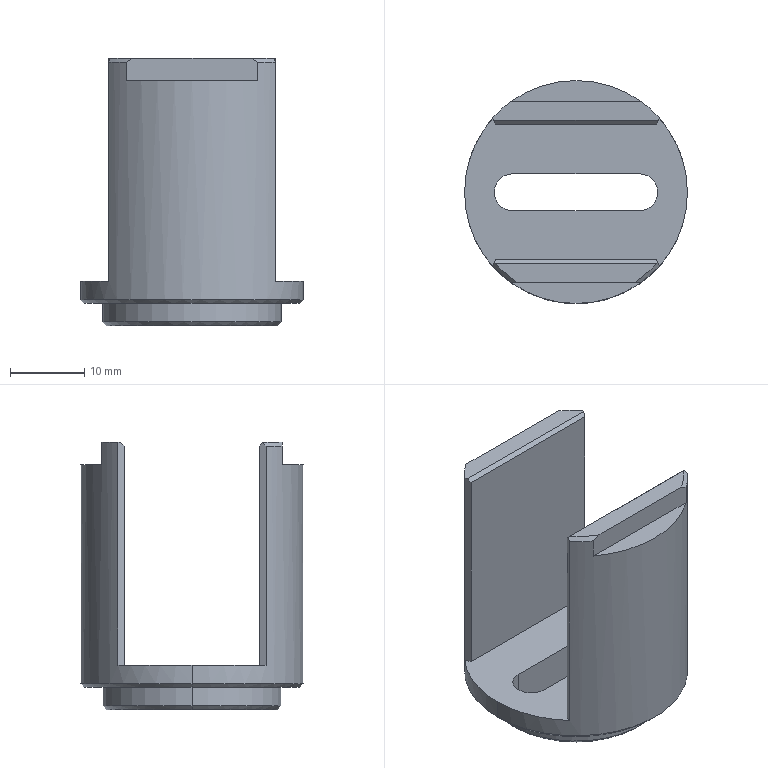Part | Creo | features CURVE 5, CHAMFER 3, DATUM PLANE 3, PROTRUSION 3, CUT 2, COORDINATE SYSTEM 1 | 1 solid | 31 faces | box 30 x 30 x 36 mm | volume 8414 mm3 | plane 19 | cylinder 6 | cone 6 | commonest cylinder face diameters 5 x2 24 x2 30 x2
STEP:
#1=CARTESIAN_POINT('',(0.,0.,0.));
#2=DIRECTION('',(0.,0.,1.));
#3=DIRECTION('',(1.,0.,0.));
#4=AXIS2_PLACEMENT_3D('',#1,#2,#3);
#5=CARTESIAN_POINT('',(-14.5,0.,0.));
#6=VERTEX_POINT('',#5);
#7=CARTESIAN_POINT('',(14.5,0.,0.));
#8=VERTEX_POINT('',#7);
#9=CARTESIAN_POINT('',(0.,0.,0.));
#10=DIRECTION('',(0.,0.,-1.));
#11=DIRECTION('',(-1.,0.,0.));
#12=AXIS2_PLACEMENT_3D('',#9,#10,#11);
#13=CIRCLE('',#12,14.5);
#14=EDGE_CURVE('',#6,#8,#13,.T.);
#15=ORIENTED_EDGE('',*,*,#14,.F.);
#16=CARTESIAN_POINT('',(0.,0.,0.));
#17=DIRECTION('',(0.,0.,-1.));
#18=DIRECTION('',(1.,0.,0.));
#19=AXIS2_PLACEMENT_3D('',#16,#17,#18);
#20=CIRCLE('',#19,14.5);
#21=EDGE_CURVE('',#8,#6,#20,.T.);
#22=ORIENTED_EDGE('',*,*,#21,.F.);
#23=EDGE_LOOP('',(#15,#22));
#24=FACE_OUTER_BOUND('',#23,.F.);
#25=CARTESIAN_POINT('',(12.,0.,0.));
#26=VERTEX_POINT('',#25);
#27=CARTESIAN_POINT('',(-12.,0.,0.));
#28=VERTEX_POINT('',#27);
#29=CARTESIAN_POINT('',(0.,0.,0.));
#30=DIRECTION('',(0.,0.,-1.));
#31=DIRECTION('',(1.,0.,0.));
#32=AXIS2_PLACEMENT_3D('',#29,#30,#31);
#33=CIRCLE('',#32,12.);
#34=EDGE_CURVE('',#26,#28,#33,.T.);
#35=ORIENTED_EDGE('',*,*,#34,.T.);
#36=CARTESIAN_POINT('',(0.,0.,0.));
#37=DIRECTION('',(0.,0.,-1.));
#38=DIRECTION('',(-1.,0.,0.));
#39=AXIS2_PLACEMENT_3D('',#36,#37,#38);
#40=CIRCLE('',#39,12.);
#41=EDGE_CURVE('',#28,#26,#40,.T.);
#42=ORIENTED_EDGE('',*,*,#41,.T.);
#43=EDGE_LOOP('',(#35,#42));
#44=FACE_BOUND('',#43,.F.);
#45=CARTESIAN_POINT('',(0.,0.,0.));
#46=DIRECTION('',(0.,0.,1.));
#47=DIRECTION('',(1.,0.,0.));
#48=AXIS2_PLACEMENT_3D('',#45,#46,#47);
#49=PLANE('',#48);
#50=ADVANCED_FACE('',(#24,#44),#49,.F.);
#51=CARTESIAN_POINT('',(12.,0.,-2.5));
#52=VERTEX_POINT('',#51);
#53=CARTESIAN_POINT('',(-12.,0.,-2.5));
#54=VERTEX_POINT('',#53);
#55=CARTESIAN_POINT('',(0.,0.,-2.5));
#56=DIRECTION('',(0.,0.,-1.));
#57=DIRECTION('',(1.,0.,0.));
#58=AXIS2_PLACEMENT_3D('',#55,#56,#57);
#59=CIRCLE('',#58,12.);
#60=EDGE_CURVE('',#52,#54,#59,.T.);
#61=ORIENTED_EDGE('',*,*,#60,.T.);
#62=CARTESIAN_POINT('',(-12.,0.,0.));
#63=DIRECTION('',(0.,0.000000001,-1.));
#64=VECTOR('',#63,2.5);
#65=LINE('',#62,#64);
#66=EDGE_CURVE('',#28,#54,#65,.T.);
#67=ORIENTED_EDGE('',*,*,#66,.F.);
#68=ORIENTED_EDGE('',*,*,#34,.F.);
#69=CARTESIAN_POINT('',(12.,0.,0.));
#70=DIRECTION('',(0.,-0.000000001,-1.));
#71=VECTOR('',#70,2.5);
#72=LINE('',#69,#71);
#73=EDGE_CURVE('',#26,#52,#72,.T.);
#74=ORIENTED_EDGE('',*,*,#73,.T.);
#75=EDGE_LOOP('',(#61,#67,#68,#74));
#76=FACE_OUTER_BOUND('',#75,.F.);
#77=CARTESIAN_POINT('',(0.,0.,0.));
#78=DIRECTION('',(0.,0.,-1.));
#79=DIRECTION('',(1.,0.,0.));
#80=AXIS2_PLACEMENT_3D('',#77,#78,#79);
#81=CYLINDRICAL_SURFACE('',#80,12.);
#82=ADVANCED_FACE('',(#76),#81,.T.);
#83=CARTESIAN_POINT('',(11.5,0.,-3.));
#84=VERTEX_POINT('',#83);
#85=CARTESIAN_POINT('',(-11.5,0.,-3.));
#86=VERTEX_POINT('',#85);
#87=CARTESIAN_POINT('',(0.,0.,-3.));
#88=DIRECTION('',(0.,0.,-1.));
#89=DIRECTION('',(1.,0.,0.));
#90=AXIS2_PLACEMENT_3D('',#87,#88,#89);
#91=CIRCLE('',#90,11.5);
#92=EDGE_CURVE('',#84,#86,#91,.T.);
#93=ORIENTED_EDGE('',*,*,#92,.T.);
#94=CARTESIAN_POINT('',(-11.5,0.000000003,-3.));
#95=DIRECTION('',(-0.7071,-0.000000001,0.7071));
#96=VECTOR('',#95,0.7071);
#97=LINE('',#94,#96);
#98=EDGE_CURVE('',#86,#54,#97,.T.);
#99=ORIENTED_EDGE('',*,*,#98,.T.);
#100=ORIENTED_EDGE('',*,*,#60,.F.);
#101=CARTESIAN_POINT('',(11.5,-0.000000003,-3.));
#102=DIRECTION('',(0.7071,0.000000001,0.7071));
#103=VECTOR('',#102,0.7071);
#104=LINE('',#101,#103);
#105=EDGE_CURVE('',#84,#52,#104,.T.);
#106=ORIENTED_EDGE('',*,*,#105,.F.);
#107=EDGE_LOOP('',(#93,#99,#100,#106));
#108=FACE_OUTER_BOUND('',#107,.F.);
#109=CARTESIAN_POINT('',(0.,0.,-2.75));
#110=DIRECTION('',(0.,0.,1.));
#111=DIRECTION('',(0.,-1.,0.));
#112=AXIS2_PLACEMENT_3D('',#109,#110,#111);
#113=CONICAL_SURFACE('',#112,11.75,45.);
#114=ADVANCED_FACE('',(#108),#113,.T.);
#115=CARTESIAN_POINT('',(0.,0.,-3.));
#116=DIRECTION('',(0.,0.,-1.));
#117=DIRECTION('',(-1.,0.,0.));
#118=AXIS2_PLACEMENT_3D('',#115,#116,#117);
#119=CIRCLE('',#118,11.5);
#120=EDGE_CURVE('',#86,#84,#119,.T.);
#121=ORIENTED_EDGE('',*,*,#120,.F.);
#122=ORIENTED_EDGE('',*,*,#92,.F.);
#123=EDGE_LOOP('',(#121,#122));
#124=FACE_OUTER_BOUND('',#123,.F.);
#125=CARTESIAN_POINT('',(8.5,2.5,-3.));
#126=VERTEX_POINT('',#125);
#127=CARTESIAN_POINT('',(8.5,-2.5,-3.));
#128=VERTEX_POINT('',#127);
#129=CARTESIAN_POINT('',(8.5,0.,-3.));
#130=DIRECTION('',(0.,0.,-1.));
#131=DIRECTION('',(0.,1.,0.));
#132=AXIS2_PLACEMENT_3D('',#129,#130,#131);
#133=CIRCLE('',#132,2.5);
#134=EDGE_CURVE('',#126,#128,#133,.T.);
#135=ORIENTED_EDGE('',*,*,#134,.T.);
#136=CARTESIAN_POINT('',(-8.5,-2.5,-3.));
#137=VERTEX_POINT('',#136);
#138=CARTESIAN_POINT('',(8.5,-2.5,-3.));
#139=DIRECTION('',(-1.,0.,0.));
#140=VECTOR('',#139,17.);
#141=LINE('',#138,#140);
#142=EDGE_CURVE('',#128,#137,#141,.T.);
#143=ORIENTED_EDGE('',*,*,#142,.T.);
#144=CARTESIAN_POINT('',(-8.5,2.5,-3.));
#145=VERTEX_POINT('',#144);
#146=CARTESIAN_POINT('',(-8.5,0.,-3.));
#147=DIRECTION('',(0.,0.,-1.));
#148=DIRECTION('',(0.,-1.,0.));
#149=AXIS2_PLACEMENT_3D('',#146,#147,#148);
#150=CIRCLE('',#149,2.5);
#151=EDGE_CURVE('',#137,#145,#150,.T.);
#152=ORIENTED_EDGE('',*,*,#151,.T.);
#153=CARTESIAN_POINT('',(-8.5,2.5,-3.));
#154=DIRECTION('',(1.,0.,0.));
#155=VECTOR('',#154,17.);
#156=LINE('',#153,#155);
#157=EDGE_CURVE('',#145,#126,#156,.T.);
#158=ORIENTED_EDGE('',*,*,#157,.T.);
#159=EDGE_LOOP('',(#135,#143,#152,#158));
#160=FACE_BOUND('',#159,.F.);
#161=CARTESIAN_POINT('',(0.,0.,-3.));
#162=DIRECTION('',(0.,0.,-1.));
#163=DIRECTION('',(1.,0.,0.));
#164=AXIS2_PLACEMENT_3D('',#161,#162,#163);
#165=PLANE('',#164);
#166=ADVANCED_FACE('',(#124,#160),#165,.T.);
#167=ORIENTED_EDGE('',*,*,#120,.T.);
#168=ORIENTED_EDGE('',*,*,#105,.T.);
#169=CARTESIAN_POINT('',(0.,0.,-2.5));
#170=DIRECTION('',(0.,0.,-1.));
#171=DIRECTION('',(-1.,0.,0.));
#172=AXIS2_PLACEMENT_3D('',#169,#170,#171);
#173=CIRCLE('',#172,12.);
#174=EDGE_CURVE('',#54,#52,#173,.T.);
#175=ORIENTED_EDGE('',*,*,#174,.F.);
#176=ORIENTED_EDGE('',*,*,#98,.F.);
#177=EDGE_LOOP('',(#167,#168,#175,#176));
#178=FACE_OUTER_BOUND('',#177,.F.);
#179=CARTESIAN_POINT('',(0.,0.,-2.75));
#180=DIRECTION('',(0.,0.,1.));
#181=DIRECTION('',(0.,-1.,0.));
#182=AXIS2_PLACEMENT_3D('',#179,#180,#181);
#183=CONICAL_SURFACE('',#182,11.75,45.);
#184=ADVANCED_FACE('',(#178),#183,.T.);
#185=ORIENTED_EDGE('',*,*,#174,.T.);
#186=ORIENTED_EDGE('',*,*,#73,.F.);
#187=ORIENTED_EDGE('',*,*,#41,.F.);
#188=ORIENTED_EDGE('',*,*,#66,.T.);
#189=EDGE_LOOP('',(#185,#186,#187,#188));
#190=FACE_OUTER_BOUND('',#189,.F.);
#191=CARTESIAN_POINT('',(0.,0.,0.));
#192=DIRECTION('',(0.,0.,-1.));
#193=DIRECTION('',(1.,0.,0.));
#194=AXIS2_PLACEMENT_3D('',#191,#192,#193);
#195=CYLINDRICAL_SURFACE('',#194,12.);
#196=ADVANCED_FACE('',(#190),#195,.T.);
#197=CARTESIAN_POINT('',(8.5,2.5,3.));
#198=VERTEX_POINT('',#197);
#199=CARTESIAN_POINT('',(8.5,-2.5,3.));
#200=VERTEX_POINT('',#199);
#201=CARTESIAN_POINT('',(8.5,0.,3.));
#202=DIRECTION('',(0.,0.,-1.));
#203=DIRECTION('',(0.,1.,0.));
#204=AXIS2_PLACEMENT_3D('',#201,#202,#203);
#205=CIRCLE('',#204,2.5);
#206=EDGE_CURVE('',#198,#200,#205,.T.);
#207=ORIENTED_EDGE('',*,*,#206,.T.);
#208=CARTESIAN_POINT('',(8.5,-2.5,-3.));
#209=DIRECTION('',(0.,0.,1.));
#210=VECTOR('',#209,6.);
#211=LINE('',#208,#210);
#212=EDGE_CURVE('',#128,#200,#211,.T.);
#213=ORIENTED_EDGE('',*,*,#212,.F.);
#214=ORIENTED_EDGE('',*,*,#134,.F.);
#215=CARTESIAN_POINT('',(8.5,2.5,-3.));
#216=DIRECTION('',(0.,0.,1.));
#217=VECTOR('',#216,6.);
#218=LINE('',#215,#217);
#219=EDGE_CURVE('',#126,#198,#218,.T.);
#220=ORIENTED_EDGE('',*,*,#219,.T.);
#221=EDGE_LOOP('',(#207,#213,#214,#220));
#222=FACE_OUTER_BOUND('',#221,.F.);
#223=CARTESIAN_POINT('',(8.5,0.,-3.));
#224=DIRECTION('',(0.,0.,-1.));
#225=DIRECTION('',(-1.,0.,0.));
#226=AXIS2_PLACEMENT_3D('',#223,#224,#225);
#227=CYLINDRICAL_SURFACE('',#226,2.5);
#228=ADVANCED_FACE('',(#222),#227,.F.);
#229=CARTESIAN_POINT('',(15.,0.,3.));
#230=VERTEX_POINT('',#229);
#231=CARTESIAN_POINT('',(11.214,-9.962,3.));
#232=VERTEX_POINT('',#231);
#233=CARTESIAN_POINT('',(0.,0.,3.));
#234=DIRECTION('',(0.,0.,-1.));
#235=DIRECTION('',(1.,0.,0.));
#236=AXIS2_PLACEMENT_3D('',#233,#234,#235);
#237=CIRCLE('',#236,15.);
#238=EDGE_CURVE('',#230,#232,#237,.T.);
#239=ORIENTED_EDGE('',*,*,#238,.T.);
#240=CARTESIAN_POINT('',(10.84,-9.13,3.));
#241=VERTEX_POINT('',#240);
#242=CARTESIAN_POINT('',(10.84,-9.13,3.));
#243=DIRECTION('',(0.4098,-0.9122,0.));
#244=VECTOR('',#243,0.9122);
#245=LINE('',#242,#244);
#246=EDGE_CURVE('',#241,#232,#245,.T.);
#247=ORIENTED_EDGE('',*,*,#246,.F.);
#248=CARTESIAN_POINT('',(-10.84,-9.13,3.));
#249=VERTEX_POINT('',#248);
#250=CARTESIAN_POINT('',(-10.84,-9.13,3.));
#251=DIRECTION('',(1.,0.,0.));
#252=VECTOR('',#251,21.681);
#253=LINE('',#250,#252);
#254=EDGE_CURVE('',#249,#241,#253,.T.);
#255=ORIENTED_EDGE('',*,*,#254,.F.);
#256=CARTESIAN_POINT('',(-11.214,-9.962,3.));
#257=VERTEX_POINT('',#256);
#258=CARTESIAN_POINT('',(-11.214,-9.962,3.));
#259=DIRECTION('',(0.4098,0.9122,0.));
#260=VECTOR('',#259,0.9122);
#261=LINE('',#258,#260);
#262=EDGE_CURVE('',#257,#249,#261,.T.);
#263=ORIENTED_EDGE('',*,*,#262,.F.);
#264=CARTESIAN_POINT('',(-15.,0.,3.));
#265=VERTEX_POINT('',#264);
#266=CARTESIAN_POINT('',(0.,0.,3.));
#267=DIRECTION('',(0.,0.,-1.));
#268=DIRECTION('',(-0.7476,-0.6641,0.));
#269=AXIS2_PLACEMENT_3D('',#266,#267,#268);
#270=CIRCLE('',#269,15.);
#271=EDGE_CURVE('',#257,#265,#270,.T.);
#272=ORIENTED_EDGE('',*,*,#271,.T.);
#273=CARTESIAN_POINT('',(-11.214,9.962,3.));
#274=VERTEX_POINT('',#273);
#275=CARTESIAN_POINT('',(0.,0.,3.));
#276=DIRECTION('',(0.,0.,-1.));
#277=DIRECTION('',(-1.,0.,0.));
#278=AXIS2_PLACEMENT_3D('',#275,#276,#277);
#279=CIRCLE('',#278,15.);
#280=EDGE_CURVE('',#265,#274,#279,.T.);
#281=ORIENTED_EDGE('',*,*,#280,.T.);
#282=CARTESIAN_POINT('',(-10.84,9.13,3.));
#283=VERTEX_POINT('',#282);
#284=CARTESIAN_POINT('',(-10.84,9.13,3.));
#285=DIRECTION('',(-0.4098,0.9122,0.));
#286=VECTOR('',#285,0.9122);
#287=LINE('',#284,#286);
#288=EDGE_CURVE('',#283,#274,#287,.T.);
#289=ORIENTED_EDGE('',*,*,#288,.F.);
#290=CARTESIAN_POINT('',(10.84,9.13,3.));
#291=VERTEX_POINT('',#290);
#292=CARTESIAN_POINT('',(10.84,9.13,3.));
#293=DIRECTION('',(-1.,0.,0.));
#294=VECTOR('',#293,21.681);
#295=LINE('',#292,#294);
#296=EDGE_CURVE('',#291,#283,#295,.T.);
#297=ORIENTED_EDGE('',*,*,#296,.F.);
#298=CARTESIAN_POINT('',(11.214,9.962,3.));
#299=VERTEX_POINT('',#298);
#300=CARTESIAN_POINT('',(11.214,9.962,3.));
#301=DIRECTION('',(-0.4098,-0.9122,0.));
#302=VECTOR('',#301,0.9122);
#303=LINE('',#300,#302);
#304=EDGE_CURVE('',#299,#291,#303,.T.);
#305=ORIENTED_EDGE('',*,*,#304,.F.);
#306=CARTESIAN_POINT('',(0.,0.,3.));
#307=DIRECTION('',(0.,0.,-1.));
#308=DIRECTION('',(0.7476,0.6641,0.));
#309=AXIS2_PLACEMENT_3D('',#306,#307,#308);
#310=CIRCLE('',#309,15.);
#311=EDGE_CURVE('',#299,#230,#310,.T.);
#312=ORIENTED_EDGE('',*,*,#311,.T.);
#313=EDGE_LOOP('',(#239,#247,#255,#263,#272,#281,#289,#297,#305,#312));
#314=FACE_OUTER_BOUND('',#313,.F.);
#315=ORIENTED_EDGE('',*,*,#206,.F.);
#316=CARTESIAN_POINT('',(-8.5,2.5,3.));
#317=VERTEX_POINT('',#316);
#318=CARTESIAN_POINT('',(-8.5,2.5,3.));
#319=DIRECTION('',(1.,0.,0.));
#320=VECTOR('',#319,17.);
#321=LINE('',#318,#320);
#322=EDGE_CURVE('',#317,#198,#321,.T.);
#323=ORIENTED_EDGE('',*,*,#322,.F.);
#324=CARTESIAN_POINT('',(-8.5,-2.5,3.));
#325=VERTEX_POINT('',#324);
#326=CARTESIAN_POINT('',(-8.5,0.,3.));
#327=DIRECTION('',(0.,0.,-1.));
#328=DIRECTION('',(0.,-1.,0.));
#329=AXIS2_PLACEMENT_3D('',#326,#327,#328);
#330=CIRCLE('',#329,2.5);
#331=EDGE_CURVE('',#325,#317,#330,.T.);
#332=ORIENTED_EDGE('',*,*,#331,.F.);
#333=CARTESIAN_POINT('',(8.5,-2.5,3.));
#334=DIRECTION('',(-1.,0.,0.));
#335=VECTOR('',#334,17.);
#336=LINE('',#333,#335);
#337=EDGE_CURVE('',#200,#325,#336,.T.);
#338=ORIENTED_EDGE('',*,*,#337,.F.);
#339=EDGE_LOOP('',(#315,#323,#332,#338));
#340=FACE_BOUND('',#339,.F.);
#341=CARTESIAN_POINT('',(0.,0.,3.));
#342=DIRECTION('',(0.,0.,1.));
#343=DIRECTION('',(1.,0.,0.));
#344=AXIS2_PLACEMENT_3D('',#341,#342,#343);
#345=PLANE('',#344);
#346=ADVANCED_FACE('',(#314,#340),#345,.T.);
#347=CARTESIAN_POINT('',(-8.824,-12.13,30.));
#348=VERTEX_POINT('',#347);
#349=CARTESIAN_POINT('',(8.824,-12.13,30.));
#350=VERTEX_POINT('',#349);
#351=CARTESIAN_POINT('',(0.,0.,30.));
#352=DIRECTION('',(0.,0.,1.));
#353=DIRECTION('',(-0.5883,-0.8087,0.));
#354=AXIS2_PLACEMENT_3D('',#351,#352,#353);
#355=CIRCLE('',#354,15.);
#356=EDGE_CURVE('',#348,#350,#355,.T.);
#357=ORIENTED_EDGE('',*,*,#356,.T.);
#358=CARTESIAN_POINT('',(8.824,-12.13,32.5));
#359=VERTEX_POINT('',#358);
#360=CARTESIAN_POINT('',(8.824,-12.13,30.));
#361=DIRECTION('',(0.,0.,1.));
#362=VECTOR('',#361,2.5);
#363=LINE('',#360,#362);
#364=EDGE_CURVE('',#350,#359,#363,.T.);
#365=ORIENTED_EDGE('',*,*,#364,.T.);
#366=CARTESIAN_POINT('',(11.214,-9.962,32.5));
#367=VERTEX_POINT('',#366);
#368=CARTESIAN_POINT('',(-0.000000704,-0.000000597,32.5));
#369=DIRECTION('',(0.,0.,-1.));
#370=DIRECTION('',(0.7476,-0.6641,0.));
#371=AXIS2_PLACEMENT_3D('',#368,#369,#370);
#372=CIRCLE('',#371,15.);
#373=EDGE_CURVE('',#367,#359,#372,.T.);
#374=ORIENTED_EDGE('',*,*,#373,.F.);
#375=CARTESIAN_POINT('',(11.214,-9.962,32.5));
#376=DIRECTION('',(0.,0.,-1.));
#377=VECTOR('',#376,29.5);
#378=LINE('',#375,#377);
#379=EDGE_CURVE('',#367,#232,#378,.T.);
#380=ORIENTED_EDGE('',*,*,#379,.T.);
#381=ORIENTED_EDGE('',*,*,#238,.F.);
#382=CARTESIAN_POINT('',(15.,0.,0.5));
#383=VERTEX_POINT('',#382);
#384=CARTESIAN_POINT('',(15.,0.000000002,0.5));
#385=DIRECTION('',(0.,-0.000000001,1.));
#386=VECTOR('',#385,2.5);
#387=LINE('',#384,#386);
#388=EDGE_CURVE('',#383,#230,#387,.T.);
#389=ORIENTED_EDGE('',*,*,#388,.F.);
#390=CARTESIAN_POINT('',(-15.,0.,0.5));
#391=VERTEX_POINT('',#390);
#392=CARTESIAN_POINT('',(0.,0.,0.5));
#393=DIRECTION('',(0.,0.,-1.));
#394=DIRECTION('',(1.,0.,0.));
#395=AXIS2_PLACEMENT_3D('',#392,#393,#394);
#396=CIRCLE('',#395,15.);
#397=EDGE_CURVE('',#383,#391,#396,.T.);
#398=ORIENTED_EDGE('',*,*,#397,.T.);
#399=CARTESIAN_POINT('',(-15.,-0.000000002,0.5));
#400=DIRECTION('',(0.,0.000000001,1.));
#401=VECTOR('',#400,2.5);
#402=LINE('',#399,#401);
#403=EDGE_CURVE('',#391,#265,#402,.T.);
#404=ORIENTED_EDGE('',*,*,#403,.T.);
#405=ORIENTED_EDGE('',*,*,#271,.F.);
#406=CARTESIAN_POINT('',(-11.214,-9.962,32.5));
#407=VERTEX_POINT('',#406);
#408=CARTESIAN_POINT('',(-11.214,-9.962,32.5));
#409=DIRECTION('',(0.,0.,-1.));
#410=VECTOR('',#409,29.5);
#411=LINE('',#408,#410);
#412=EDGE_CURVE('',#407,#257,#411,.T.);
#413=ORIENTED_EDGE('',*,*,#412,.F.);
#414=CARTESIAN_POINT('',(-8.824,-12.13,32.5));
#415=VERTEX_POINT('',#414);
#416=CARTESIAN_POINT('',(-0.000000704,-0.000000597,32.5));
#417=DIRECTION('',(0.,0.,-1.));
#418=DIRECTION('',(-0.5883,-0.8087,0.));
#419=AXIS2_PLACEMENT_3D('',#416,#417,#418);
#420=CIRCLE('',#419,15.);
#421=EDGE_CURVE('',#415,#407,#420,.T.);
#422=ORIENTED_EDGE('',*,*,#421,.F.);
#423=CARTESIAN_POINT('',(-8.824,-12.13,30.));
#424=DIRECTION('',(0.,0.,1.));
#425=VECTOR('',#424,2.5);
#426=LINE('',#423,#425);
#427=EDGE_CURVE('',#348,#415,#426,.T.);
#428=ORIENTED_EDGE('',*,*,#427,.F.);
#429=EDGE_LOOP('',(#357,#365,#374,#380,#381,#389,#398,#404,#405,#413,#422,#428));
#430=FACE_OUTER_BOUND('',#429,.F.);
#431=CARTESIAN_POINT('',(0.,0.,0.));
#432=DIRECTION('',(0.,0.,1.));
#433=DIRECTION('',(1.,0.,0.));
#434=AXIS2_PLACEMENT_3D('',#431,#432,#433);
#435=CYLINDRICAL_SURFACE('',#434,15.);
#436=ADVANCED_FACE('',(#430),#435,.T.);
#437=CARTESIAN_POINT('',(8.824,12.13,30.));
#438=VERTEX_POINT('',#437);
#439=CARTESIAN_POINT('',(-8.824,12.13,30.));
#440=VERTEX_POINT('',#439);
#441=CARTESIAN_POINT('',(0.,0.,30.));
#442=DIRECTION('',(0.,0.,1.));
#443=DIRECTION('',(0.5883,0.8087,0.));
#444=AXIS2_PLACEMENT_3D('',#441,#442,#443);
#445=CIRCLE('',#444,15.);
#446=EDGE_CURVE('',#438,#440,#445,.T.);
#447=ORIENTED_EDGE('',*,*,#446,.F.);
#448=CARTESIAN_POINT('',(-8.824,12.13,30.));
#449=DIRECTION('',(1.,0.,0.));
#450=VECTOR('',#449,17.648);
#451=LINE('',#448,#450);
#452=EDGE_CURVE('',#440,#438,#451,.T.);
#453=ORIENTED_EDGE('',*,*,#452,.F.);
#454=EDGE_LOOP('',(#447,#453));
#455=FACE_OUTER_BOUND('',#454,.F.);
#456=CARTESIAN_POINT('',(0.,0.,30.));
#457=DIRECTION('',(0.,0.,1.));
#458=DIRECTION('',(1.,0.,0.));
#459=AXIS2_PLACEMENT_3D('',#456,#457,#458);
#460=PLANE('',#459);
#461=ADVANCED_FACE('',(#455),#460,.T.);
#462=ORIENTED_EDGE('',*,*,#356,.F.);
#463=CARTESIAN_POINT('',(8.824,-12.13,30.));
#464=DIRECTION('',(-1.,0.,0.));
#465=VECTOR('',#464,17.648);
#466=LINE('',#463,#465);
#467=EDGE_CURVE('',#350,#348,#466,.T.);
#468=ORIENTED_EDGE('',*,*,#467,.F.);
#469=EDGE_LOOP('',(#462,#468));
#470=FACE_OUTER_BOUND('',#469,.F.);
#471=CARTESIAN_POINT('',(0.,0.,30.));
#472=DIRECTION('',(0.,0.,1.));
#473=DIRECTION('',(1.,0.,0.));
#474=AXIS2_PLACEMENT_3D('',#471,#472,#473);
#475=PLANE('',#474);
#476=ADVANCED_FACE('',(#470),#475,.T.);
#477=ORIENTED_EDGE('',*,*,#446,.T.);
#478=CARTESIAN_POINT('',(-8.824,12.13,33.));
#479=VERTEX_POINT('',#478);
#480=CARTESIAN_POINT('',(-8.824,12.13,30.));
#481=DIRECTION('',(0.,0.,1.));
#482=VECTOR('',#481,3.);
#483=LINE('',#480,#482);
#484=EDGE_CURVE('',#440,#479,#483,.T.);
#485=ORIENTED_EDGE('',*,*,#484,.T.);
#486=CARTESIAN_POINT('',(-11.214,9.962,33.));
#487=VERTEX_POINT('',#486);
#488=CARTESIAN_POINT('',(0.,0.,33.));
#489=DIRECTION('',(0.,0.,1.));
#490=DIRECTION('',(-0.5883,0.8087,0.));
#491=AXIS2_PLACEMENT_3D('',#488,#489,#490);
#492=CIRCLE('',#491,15.);
#493=EDGE_CURVE('',#479,#487,#492,.T.);
#494=ORIENTED_EDGE('',*,*,#493,.T.);
#495=CARTESIAN_POINT('',(-11.214,9.962,33.));
#496=DIRECTION('',(0.,0.,-1.));
#497=VECTOR('',#496,30.);
#498=LINE('',#495,#497);
#499=EDGE_CURVE('',#487,#274,#498,.T.);
#500=ORIENTED_EDGE('',*,*,#499,.T.);
#501=ORIENTED_EDGE('',*,*,#280,.F.);
#502=ORIENTED_EDGE('',*,*,#403,.F.);
#503=CARTESIAN_POINT('',(0.,0.,0.5));
#504=DIRECTION('',(0.,0.,-1.));
#505=DIRECTION('',(-1.,0.,0.));
#506=AXIS2_PLACEMENT_3D('',#503,#504,#505);
#507=CIRCLE('',#506,15.);
#508=EDGE_CURVE('',#391,#383,#507,.T.);
#509=ORIENTED_EDGE('',*,*,#508,.T.);
#510=ORIENTED_EDGE('',*,*,#388,.T.);
#511=ORIENTED_EDGE('',*,*,#311,.F.);
#512=CARTESIAN_POINT('',(11.214,9.962,33.));
#513=VERTEX_POINT('',#512);
#514=CARTESIAN_POINT('',(11.214,9.962,33.));
#515=DIRECTION('',(0.,0.,-1.));
#516=VECTOR('',#515,30.);
#517=LINE('',#514,#516);
#518=EDGE_CURVE('',#513,#299,#517,.T.);
#519=ORIENTED_EDGE('',*,*,#518,.F.);
#520=CARTESIAN_POINT('',(8.824,12.13,33.));
#521=VERTEX_POINT('',#520);
#522=CARTESIAN_POINT('',(0.,0.,33.));
#523=DIRECTION('',(0.,0.,1.));
#524=DIRECTION('',(0.7476,0.6641,0.));
#525=AXIS2_PLACEMENT_3D('',#522,#523,#524);
#526=CIRCLE('',#525,15.);
#527=EDGE_CURVE('',#513,#521,#526,.T.);
#528=ORIENTED_EDGE('',*,*,#527,.T.);
#529=CARTESIAN_POINT('',(8.824,12.13,30.));
#530=DIRECTION('',(0.,0.,1.));
#531=VECTOR('',#530,3.);
#532=LINE('',#529,#531);
#533=EDGE_CURVE('',#438,#521,#532,.T.);
#534=ORIENTED_EDGE('',*,*,#533,.F.);
#535=EDGE_LOOP('',(#477,#485,#494,#500,#501,#502,#509,#510,#511,#519,#528,#534));
#536=FACE_OUTER_BOUND('',#535,.F.);
#537=CARTESIAN_POINT('',(0.,0.,0.));
#538=DIRECTION('',(0.,0.,1.));
#539=DIRECTION('',(1.,0.,0.));
#540=AXIS2_PLACEMENT_3D('',#537,#538,#539);
#541=CYLINDRICAL_SURFACE('',#540,15.);
#542=ADVANCED_FACE('',(#536),#541,.T.);
#543=ORIENTED_EDGE('',*,*,#533,.T.);
#544=CARTESIAN_POINT('',(-8.824,12.13,33.));
#545=DIRECTION('',(1.,0.,0.));
#546=VECTOR('',#545,17.648);
#547=LINE('',#544,#546);
#548=EDGE_CURVE('',#479,#521,#547,.T.);
#549=ORIENTED_EDGE('',*,*,#548,.F.);
#550=ORIENTED_EDGE('',*,*,#484,.F.);
#551=ORIENTED_EDGE('',*,*,#452,.T.);
#552=EDGE_LOOP('',(#543,#549,#550,#551));
#553=FACE_OUTER_BOUND('',#552,.F.);
#554=CARTESIAN_POINT('',(-8.824,12.13,33.));
#555=DIRECTION('',(0.,-1.,0.));
#556=DIRECTION('',(1.,0.,0.));
#557=AXIS2_PLACEMENT_3D('',#554,#555,#556);
#558=PLANE('',#557);
#559=ADVANCED_FACE('',(#553),#558,.F.);
#560=ORIENTED_EDGE('',*,*,#548,.T.);
#561=ORIENTED_EDGE('',*,*,#527,.F.);
#562=CARTESIAN_POINT('',(11.065,9.63,33.));
#563=VERTEX_POINT('',#562);
#564=CARTESIAN_POINT('',(11.065,9.63,33.));
#565=DIRECTION('',(0.4098,0.9122,0.));
#566=VECTOR('',#565,0.364);
#567=LINE('',#564,#566);
#568=EDGE_CURVE('',#563,#513,#567,.T.);
#569=ORIENTED_EDGE('',*,*,#568,.F.);
#570=CARTESIAN_POINT('',(-11.065,9.63,33.));
#571=VERTEX_POINT('',#570);
#572=CARTESIAN_POINT('',(11.065,9.63,33.));
#573=DIRECTION('',(-1.,0.,0.));
#574=VECTOR('',#573,22.13);
#575=LINE('',#572,#574);
#576=EDGE_CURVE('',#563,#571,#575,.T.);
#577=ORIENTED_EDGE('',*,*,#576,.T.);
#578=CARTESIAN_POINT('',(-11.214,9.962,33.));
#579=DIRECTION('',(0.4098,-0.9122,0.));
#580=VECTOR('',#579,0.364);
#581=LINE('',#578,#580);
#582=EDGE_CURVE('',#487,#571,#581,.T.);
#583=ORIENTED_EDGE('',*,*,#582,.F.);
#584=ORIENTED_EDGE('',*,*,#493,.F.);
#585=EDGE_LOOP('',(#560,#561,#569,#577,#583,#584));
#586=FACE_OUTER_BOUND('',#585,.F.);
#587=CARTESIAN_POINT('',(0.,0.,33.));
#588=DIRECTION('',(0.,0.,1.));
#589=DIRECTION('',(1.,0.,0.));
#590=AXIS2_PLACEMENT_3D('',#587,#588,#589);
#591=PLANE('',#590);
#592=ADVANCED_FACE('',(#586),#591,.T.);
#593=CARTESIAN_POINT('',(7.944,-12.13,33.));
#594=VERTEX_POINT('',#593);
#595=CARTESIAN_POINT('',(-7.944,-12.13,33.));
#596=VERTEX_POINT('',#595);
#597=CARTESIAN_POINT('',(7.944,-12.13,33.));
#598=DIRECTION('',(-1.,0.,0.));
#599=VECTOR('',#598,15.889);
#600=LINE('',#597,#599);
#601=EDGE_CURVE('',#594,#596,#600,.T.);
#602=ORIENTED_EDGE('',*,*,#601,.T.);
#603=CARTESIAN_POINT('',(-10.84,-9.63,33.));
#604=VERTEX_POINT('',#603);
#605=CARTESIAN_POINT('',(-0.000000704,-0.000000597,33.));
#606=DIRECTION('',(0.,0.,1.));
#607=DIRECTION('',(-0.7476,-0.6641,0.));
#608=AXIS2_PLACEMENT_3D('',#605,#606,#607);
#609=CIRCLE('',#608,14.5);
#610=EDGE_CURVE('',#604,#596,#609,.T.);
#611=ORIENTED_EDGE('',*,*,#610,.F.);
#612=CARTESIAN_POINT('',(10.84,-9.63,33.));
#613=VERTEX_POINT('',#612);
#614=CARTESIAN_POINT('',(-10.84,-9.63,33.));
#615=DIRECTION('',(1.,0.,0.));
#616=VECTOR('',#615,21.681);
#617=LINE('',#614,#616);
#618=EDGE_CURVE('',#604,#613,#617,.T.);
#619=ORIENTED_EDGE('',*,*,#618,.T.);
#620=CARTESIAN_POINT('',(-0.000000704,-0.000000597,33.));
#621=DIRECTION('',(0.,0.,1.));
#622=DIRECTION('',(0.5479,-0.8366,0.));
#623=AXIS2_PLACEMENT_3D('',#620,#621,#622);
#624=CIRCLE('',#623,14.5);
#625=EDGE_CURVE('',#594,#613,#624,.T.);
#626=ORIENTED_EDGE('',*,*,#625,.F.);
#627=EDGE_LOOP('',(#602,#611,#619,#626));
#628=FACE_OUTER_BOUND('',#627,.F.);
#629=CARTESIAN_POINT('',(0.,0.,33.));
#630=DIRECTION('',(0.,0.,1.));
#631=DIRECTION('',(1.,0.,0.));
#632=AXIS2_PLACEMENT_3D('',#629,#630,#631);
#633=PLANE('',#632);
#634=ADVANCED_FACE('',(#628),#633,.T.);
#635=CARTESIAN_POINT('',(10.84,9.13,32.5));
#636=VERTEX_POINT('',#635);
#637=CARTESIAN_POINT('',(10.84,9.13,32.5));
#638=DIRECTION('',(0.,0.,-1.));
#639=VECTOR('',#638,29.5);
#640=LINE('',#637,#639);
#641=EDGE_CURVE('',#636,#291,#640,.T.);
#642=ORIENTED_EDGE('',*,*,#641,.F.);
#643=CARTESIAN_POINT('',(10.84,9.13,32.5));
#644=DIRECTION('',(0.3028,0.6739,0.6739));
#645=VECTOR('',#644,0.7419);
#646=LINE('',#643,#645);
#647=EDGE_CURVE('',#636,#563,#646,.T.);
#648=ORIENTED_EDGE('',*,*,#647,.T.);
#649=ORIENTED_EDGE('',*,*,#568,.T.);
#650=ORIENTED_EDGE('',*,*,#518,.T.);
#651=ORIENTED_EDGE('',*,*,#304,.T.);
#652=EDGE_LOOP('',(#642,#648,#649,#650,#651));
#653=FACE_OUTER_BOUND('',#652,.F.);
#654=CARTESIAN_POINT('',(11.027,9.546,18.));
#655=DIRECTION('',(0.9122,-0.4098,0.));
#656=DIRECTION('',(-0.4098,-0.9122,0.));
#657=AXIS2_PLACEMENT_3D('',#654,#655,#656);
#658=PLANE('',#657);
#659=ADVANCED_FACE('',(#653),#658,.T.);
#660=ORIENTED_EDGE('',*,*,#641,.T.);
#661=ORIENTED_EDGE('',*,*,#296,.T.);
#662=CARTESIAN_POINT('',(-10.84,9.13,32.5));
#663=VERTEX_POINT('',#662);
#664=CARTESIAN_POINT('',(-10.84,9.13,32.5));
#665=DIRECTION('',(0.,0.,-1.));
#666=VECTOR('',#665,29.5);
#667=LINE('',#664,#666);
#668=EDGE_CURVE('',#663,#283,#667,.T.);
#669=ORIENTED_EDGE('',*,*,#668,.F.);
#670=CARTESIAN_POINT('',(10.84,9.13,32.5));
#671=DIRECTION('',(-1.,0.,0.));
#672=VECTOR('',#671,21.681);
#673=LINE('',#670,#672);
#674=EDGE_CURVE('',#636,#663,#673,.T.);
#675=ORIENTED_EDGE('',*,*,#674,.F.);
#676=EDGE_LOOP('',(#660,#661,#669,#675));
#677=FACE_OUTER_BOUND('',#676,.F.);
#678=CARTESIAN_POINT('',(-11.901,9.13,3.));
#679=DIRECTION('',(0.,-1.,0.));
#680=DIRECTION('',(1.,0.,0.));
#681=AXIS2_PLACEMENT_3D('',#678,#679,#680);
#682=PLANE('',#681);
#683=ADVANCED_FACE('',(#677),#682,.T.);
#684=CARTESIAN_POINT('',(-10.84,9.13,32.5));
#685=DIRECTION('',(-0.3028,0.6739,0.6739));
#686=VECTOR('',#685,0.7419);
#687=LINE('',#684,#686);
#688=EDGE_CURVE('',#663,#571,#687,.T.);
#689=ORIENTED_EDGE('',*,*,#688,.F.);
#690=ORIENTED_EDGE('',*,*,#668,.T.);
#691=ORIENTED_EDGE('',*,*,#288,.T.);
#692=ORIENTED_EDGE('',*,*,#499,.F.);
#693=ORIENTED_EDGE('',*,*,#582,.T.);
#694=EDGE_LOOP('',(#689,#690,#691,#692,#693));
#695=FACE_OUTER_BOUND('',#694,.F.);
#696=CARTESIAN_POINT('',(-11.027,9.546,18.));
#697=DIRECTION('',(-0.9122,-0.4098,0.));
#698=DIRECTION('',(-0.4098,0.9122,0.));
#699=AXIS2_PLACEMENT_3D('',#696,#697,#698);
#700=PLANE('',#699);
#701=ADVANCED_FACE('',(#695),#700,.T.);
#702=ORIENTED_EDGE('',*,*,#688,.T.);
#703=ORIENTED_EDGE('',*,*,#576,.F.);
#704=ORIENTED_EDGE('',*,*,#647,.F.);
#705=ORIENTED_EDGE('',*,*,#674,.T.);
#706=EDGE_LOOP('',(#702,#703,#704,#705));
#707=FACE_OUTER_BOUND('',#706,.F.);
#708=CARTESIAN_POINT('',(0.3301,9.38,32.75));
#709=DIRECTION('',(0.,-0.7071,0.7071));
#710=DIRECTION('',(0.,0.7071,0.7071));
#711=AXIS2_PLACEMENT_3D('',#708,#709,#710);
#712=PLANE('',#711);
#713=ADVANCED_FACE('',(#707),#712,.T.);
#714=ORIENTED_EDGE('',*,*,#427,.T.);
#715=CARTESIAN_POINT('',(-7.944,-12.13,33.));
#716=CARTESIAN_POINT('',(-8.04,-12.13,32.948));
#717=CARTESIAN_POINT('',(-8.232,-12.13,32.841));
#718=CARTESIAN_POINT('',(-8.525,-12.13,32.675));
#719=CARTESIAN_POINT('',(-8.724,-12.13,32.559));
#720=CARTESIAN_POINT('',(-8.824,-12.13,32.5));
#721=B_SPLINE_CURVE_WITH_KNOTS('',3,(#715,#716,#717,#718,#719,#720),.UNSPECIFIED.,.F.,.F.,(4,1,1,4),(0.,0.3333,0.6667,1.),.UNSPECIFIED.);
#722=EDGE_CURVE('',#596,#415,#721,.T.);
#723=ORIENTED_EDGE('',*,*,#722,.F.);
#724=ORIENTED_EDGE('',*,*,#601,.F.);
#725=CARTESIAN_POINT('',(8.824,-12.13,32.5));
#726=CARTESIAN_POINT('',(8.724,-12.13,32.559));
#727=CARTESIAN_POINT('',(8.525,-12.13,32.675));
#728=CARTESIAN_POINT('',(8.232,-12.13,32.841));
#729=CARTESIAN_POINT('',(8.04,-12.13,32.948));
#730=CARTESIAN_POINT('',(7.944,-12.13,33.));
#731=B_SPLINE_CURVE_WITH_KNOTS('',3,(#725,#726,#727,#728,#729,#730),.UNSPECIFIED.,.F.,.F.,(4,1,1,4),(0.,0.3333,0.6667,1.),.UNSPECIFIED.);
#732=EDGE_CURVE('',#359,#594,#731,.T.);
#733=ORIENTED_EDGE('',*,*,#732,.F.);
#734=ORIENTED_EDGE('',*,*,#364,.F.);
#735=ORIENTED_EDGE('',*,*,#467,.T.);
#736=EDGE_LOOP('',(#714,#723,#724,#733,#734,#735));
#737=FACE_OUTER_BOUND('',#736,.F.);
#738=CARTESIAN_POINT('',(8.824,-12.13,33.));
#739=DIRECTION('',(0.,1.,0.));
#740=DIRECTION('',(-1.,0.,0.));
#741=AXIS2_PLACEMENT_3D('',#738,#739,#740);
#742=PLANE('',#741);
#743=ADVANCED_FACE('',(#737),#742,.F.);
#744=ORIENTED_EDGE('',*,*,#732,.T.);
#745=ORIENTED_EDGE('',*,*,#625,.T.);
#746=CARTESIAN_POINT('',(11.027,-9.545,32.915));
#747=VERTEX_POINT('',#746);
#748=CARTESIAN_POINT('',(11.027,-9.545,32.915));
#749=CARTESIAN_POINT('',(11.006,-9.555,32.925));
#750=CARTESIAN_POINT('',(10.965,-9.574,32.944));
#751=CARTESIAN_POINT('',(10.903,-9.602,32.972));
#752=CARTESIAN_POINT('',(10.861,-9.621,32.991));
#753=B_SPLINE_CURVE_WITH_KNOTS('',3,(#748,#749,#750,#751,#752,#612),.UNSPECIFIED.,.F.,.F.,(4,1,1,4),(0.,0.3333,0.6667,1.),.UNSPECIFIED.);
#754=EDGE_CURVE('',#747,#613,#753,.T.);
#755=ORIENTED_EDGE('',*,*,#754,.F.);
#756=CARTESIAN_POINT('',(11.214,-9.962,32.5));
#757=CARTESIAN_POINT('',(11.193,-9.915,32.547));
#758=CARTESIAN_POINT('',(11.151,-9.822,32.64));
#759=CARTESIAN_POINT('',(11.089,-9.683,32.778));
#760=CARTESIAN_POINT('',(11.048,-9.591,32.87));
#761=B_SPLINE_CURVE_WITH_KNOTS('',3,(#756,#757,#758,#759,#760,#746),.UNSPECIFIED.,.F.,.F.,(4,1,1,4),(0.,0.3333,0.6667,1.),.UNSPECIFIED.);
#762=EDGE_CURVE('',#367,#747,#761,.T.);
#763=ORIENTED_EDGE('',*,*,#762,.F.);
#764=ORIENTED_EDGE('',*,*,#373,.T.);
#765=EDGE_LOOP('',(#744,#745,#755,#763,#764));
#766=FACE_OUTER_BOUND('',#765,.F.);
#767=CARTESIAN_POINT('',(-0.000000704,-0.000000597,32.75));
#768=DIRECTION('',(0.,0.,-1.));
#769=DIRECTION('',(0.,-1.,0.));
#770=AXIS2_PLACEMENT_3D('',#767,#768,#769);
#771=CONICAL_SURFACE('',#770,14.75,45.);
#772=ADVANCED_FACE('',(#766),#771,.T.);
#773=ORIENTED_EDGE('',*,*,#722,.T.);
#774=ORIENTED_EDGE('',*,*,#421,.T.);
#775=CARTESIAN_POINT('',(-11.027,-9.545,32.915));
#776=VERTEX_POINT('',#775);
#777=CARTESIAN_POINT('',(-11.027,-9.545,32.915));
#778=CARTESIAN_POINT('',(-11.058,-9.614,32.847));
#779=CARTESIAN_POINT('',(-11.12,-9.752,32.71));
#780=CARTESIAN_POINT('',(-11.183,-9.892,32.57));
#781=CARTESIAN_POINT('',(-11.214,-9.962,32.5));
#782=B_SPLINE_CURVE_WITH_KNOTS('',3,(#777,#778,#779,#780,#781),.UNSPECIFIED.,.F.,.F.,(4,1,4),(0.,0.5,1.),.UNSPECIFIED.);
#783=EDGE_CURVE('',#776,#407,#782,.T.);
#784=ORIENTED_EDGE('',*,*,#783,.F.);
#785=CARTESIAN_POINT('',(-10.871,-9.616,32.986));
#786=CARTESIAN_POINT('',(-10.934,-9.588,32.958));
#787=CARTESIAN_POINT('',(-10.996,-9.56,32.93));
#788=B_SPLINE_CURVE_WITH_KNOTS('',3,(#603,#785,#786,#787,#775),.UNSPECIFIED.,.F.,.F.,(4,1,4),(0.,0.5,1.),.UNSPECIFIED.);
#789=EDGE_CURVE('',#604,#776,#788,.T.);
#790=ORIENTED_EDGE('',*,*,#789,.F.);
#791=ORIENTED_EDGE('',*,*,#610,.T.);
#792=EDGE_LOOP('',(#773,#774,#784,#790,#791));
#793=FACE_OUTER_BOUND('',#792,.F.);
#794=CARTESIAN_POINT('',(-0.000000704,-0.000000597,32.75));
#795=DIRECTION('',(0.,0.,-1.));
#796=DIRECTION('',(0.,-1.,0.));
#797=AXIS2_PLACEMENT_3D('',#794,#795,#796);
#798=CONICAL_SURFACE('',#797,14.75,45.);
#799=ADVANCED_FACE('',(#793),#798,.T.);
#800=ORIENTED_EDGE('',*,*,#789,.T.);
#801=CARTESIAN_POINT('',(-10.84,-9.13,32.5));
#802=VERTEX_POINT('',#801);
#803=CARTESIAN_POINT('',(-11.027,-9.545,32.915));
#804=DIRECTION('',(0.3028,0.6739,-0.6739));
#805=VECTOR('',#804,0.6164);
#806=LINE('',#803,#805);
#807=EDGE_CURVE('',#776,#802,#806,.T.);
#808=ORIENTED_EDGE('',*,*,#807,.T.);
#809=CARTESIAN_POINT('',(10.84,-9.13,32.5));
#810=VERTEX_POINT('',#809);
#811=CARTESIAN_POINT('',(-10.84,-9.13,32.5));
#812=DIRECTION('',(1.,0.,0.));
#813=VECTOR('',#812,21.681);
#814=LINE('',#811,#813);
#815=EDGE_CURVE('',#802,#810,#814,.T.);
#816=ORIENTED_EDGE('',*,*,#815,.T.);
#817=CARTESIAN_POINT('',(10.84,-9.13,32.5));
#818=DIRECTION('',(0.3028,-0.6739,0.6739));
#819=VECTOR('',#818,0.6164);
#820=LINE('',#817,#819);
#821=EDGE_CURVE('',#810,#747,#820,.T.);
#822=ORIENTED_EDGE('',*,*,#821,.T.);
#823=ORIENTED_EDGE('',*,*,#754,.T.);
#824=ORIENTED_EDGE('',*,*,#618,.F.);
#825=EDGE_LOOP('',(#800,#808,#816,#822,#823,#824));
#826=FACE_OUTER_BOUND('',#825,.F.);
#827=CARTESIAN_POINT('',(-0.000000704,-9.38,32.75));
#828=DIRECTION('',(0.,0.7071,0.7071));
#829=DIRECTION('',(0.,-0.7071,0.7071));
#830=AXIS2_PLACEMENT_3D('',#827,#828,#829);
#831=PLANE('',#830);
#832=ADVANCED_FACE('',(#826),#831,.T.);
#833=ORIENTED_EDGE('',*,*,#807,.F.);
#834=ORIENTED_EDGE('',*,*,#783,.T.);
#835=ORIENTED_EDGE('',*,*,#412,.T.);
#836=ORIENTED_EDGE('',*,*,#262,.T.);
#837=CARTESIAN_POINT('',(-10.84,-9.13,32.5));
#838=DIRECTION('',(0.,0.,-1.));
#839=VECTOR('',#838,29.5);
#840=LINE('',#837,#839);
#841=EDGE_CURVE('',#802,#249,#840,.T.);
#842=ORIENTED_EDGE('',*,*,#841,.F.);
#843=EDGE_LOOP('',(#833,#834,#835,#836,#842));
#844=FACE_OUTER_BOUND('',#843,.F.);
#845=CARTESIAN_POINT('',(-11.027,-9.546,17.75));
#846=DIRECTION('',(-0.9122,0.4098,0.));
#847=DIRECTION('',(0.4098,0.9122,0.));
#848=AXIS2_PLACEMENT_3D('',#845,#846,#847);
#849=PLANE('',#848);
#850=ADVANCED_FACE('',(#844),#849,.T.);
#851=CARTESIAN_POINT('',(10.84,-9.13,32.5));
#852=DIRECTION('',(0.,0.,-1.));
#853=VECTOR('',#852,29.5);
#854=LINE('',#851,#853);
#855=EDGE_CURVE('',#810,#241,#854,.T.);
#856=ORIENTED_EDGE('',*,*,#855,.F.);
#857=ORIENTED_EDGE('',*,*,#815,.F.);
#858=ORIENTED_EDGE('',*,*,#841,.T.);
#859=ORIENTED_EDGE('',*,*,#254,.T.);
#860=EDGE_LOOP('',(#856,#857,#858,#859));
#861=FACE_OUTER_BOUND('',#860,.F.);
#862=CARTESIAN_POINT('',(5.6,-9.13,3.));
#863=DIRECTION('',(0.,1.,0.));
#864=DIRECTION('',(-1.,0.,0.));
#865=AXIS2_PLACEMENT_3D('',#862,#863,#864);
#866=PLANE('',#865);
#867=ADVANCED_FACE('',(#861),#866,.T.);
#868=ORIENTED_EDGE('',*,*,#379,.F.);
#869=ORIENTED_EDGE('',*,*,#762,.T.);
#870=ORIENTED_EDGE('',*,*,#821,.F.);
#871=ORIENTED_EDGE('',*,*,#855,.T.);
#872=ORIENTED_EDGE('',*,*,#246,.T.);
#873=EDGE_LOOP('',(#868,#869,#870,#871,#872));
#874=FACE_OUTER_BOUND('',#873,.F.);
#875=CARTESIAN_POINT('',(11.027,-9.546,17.75));
#876=DIRECTION('',(0.9122,0.4098,0.));
#877=DIRECTION('',(0.4098,-0.9122,0.));
#878=AXIS2_PLACEMENT_3D('',#875,#876,#877);
#879=PLANE('',#878);
#880=ADVANCED_FACE('',(#874),#879,.T.);
#881=ORIENTED_EDGE('',*,*,#14,.T.);
#882=CARTESIAN_POINT('',(14.5,0.000000003,0.));
#883=DIRECTION('',(0.7071,-0.000000001,0.7071));
#884=VECTOR('',#883,0.7071);
#885=LINE('',#882,#884);
#886=EDGE_CURVE('',#8,#383,#885,.T.);
#887=ORIENTED_EDGE('',*,*,#886,.T.);
#888=ORIENTED_EDGE('',*,*,#508,.F.);
#889=CARTESIAN_POINT('',(-14.5,-0.000000003,0.));
#890=DIRECTION('',(-0.7071,0.000000001,0.7071));
#891=VECTOR('',#890,0.7071);
#892=LINE('',#889,#891);
#893=EDGE_CURVE('',#6,#391,#892,.T.);
#894=ORIENTED_EDGE('',*,*,#893,.F.);
#895=EDGE_LOOP('',(#881,#887,#888,#894));
#896=FACE_OUTER_BOUND('',#895,.F.);
#897=CARTESIAN_POINT('',(0.,0.,0.25));
#898=DIRECTION('',(0.,0.,1.));
#899=DIRECTION('',(0.,-1.,0.));
#900=AXIS2_PLACEMENT_3D('',#897,#898,#899);
#901=CONICAL_SURFACE('',#900,14.75,45.);
#902=ADVANCED_FACE('',(#896),#901,.T.);
#903=ORIENTED_EDGE('',*,*,#21,.T.);
#904=ORIENTED_EDGE('',*,*,#893,.T.);
#905=ORIENTED_EDGE('',*,*,#397,.F.);
#906=ORIENTED_EDGE('',*,*,#886,.F.);
#907=EDGE_LOOP('',(#903,#904,#905,#906));
#908=FACE_OUTER_BOUND('',#907,.F.);
#909=CARTESIAN_POINT('',(0.,0.,0.25));
#910=DIRECTION('',(0.,0.,1.));
#911=DIRECTION('',(0.,-1.,0.));
#912=AXIS2_PLACEMENT_3D('',#909,#910,#911);
#913=CONICAL_SURFACE('',#912,14.75,45.);
#914=ADVANCED_FACE('',(#908),#913,.T.);
#915=ORIENTED_EDGE('',*,*,#322,.T.);
#916=ORIENTED_EDGE('',*,*,#219,.F.);
#917=ORIENTED_EDGE('',*,*,#157,.F.);
#918=CARTESIAN_POINT('',(-8.5,2.5,-3.));
#919=DIRECTION('',(0.,0.,1.));
#920=VECTOR('',#919,6.);
#921=LINE('',#918,#920);
#922=EDGE_CURVE('',#145,#317,#921,.T.);
#923=ORIENTED_EDGE('',*,*,#922,.T.);
#924=EDGE_LOOP('',(#915,#916,#917,#923));
#925=FACE_OUTER_BOUND('',#924,.F.);
#926=CARTESIAN_POINT('',(-8.5,2.5,-3.));
#927=DIRECTION('',(0.,1.,0.));
#928=DIRECTION('',(1.,0.,0.));
#929=AXIS2_PLACEMENT_3D('',#926,#927,#928);
#930=PLANE('',#929);
#931=ADVANCED_FACE('',(#925),#930,.F.);
#932=ORIENTED_EDGE('',*,*,#331,.T.);
#933=ORIENTED_EDGE('',*,*,#922,.F.);
#934=ORIENTED_EDGE('',*,*,#151,.F.);
#935=CARTESIAN_POINT('',(-8.5,-2.5,-3.));
#936=DIRECTION('',(0.,0.,1.));
#937=VECTOR('',#936,6.);
#938=LINE('',#935,#937);
#939=EDGE_CURVE('',#137,#325,#938,.T.);
#940=ORIENTED_EDGE('',*,*,#939,.T.);
#941=EDGE_LOOP('',(#932,#933,#934,#940));
#942=FACE_OUTER_BOUND('',#941,.F.);
#943=CARTESIAN_POINT('',(-8.5,0.,-3.));
#944=DIRECTION('',(0.,0.,-1.));
#945=DIRECTION('',(-1.,0.,0.));
#946=AXIS2_PLACEMENT_3D('',#943,#944,#945);
#947=CYLINDRICAL_SURFACE('',#946,2.5);
#948=ADVANCED_FACE('',(#942),#947,.F.);
#949=ORIENTED_EDGE('',*,*,#337,.T.);
#950=ORIENTED_EDGE('',*,*,#939,.F.);
#951=ORIENTED_EDGE('',*,*,#142,.F.);
#952=ORIENTED_EDGE('',*,*,#212,.T.);
#953=EDGE_LOOP('',(#949,#950,#951,#952));
#954=FACE_OUTER_BOUND('',#953,.F.);
#955=CARTESIAN_POINT('',(8.5,-2.5,-3.));
#956=DIRECTION('',(0.,-1.,0.));
#957=DIRECTION('',(-1.,0.,0.));
#958=AXIS2_PLACEMENT_3D('',#955,#956,#957);
#959=PLANE('',#958);
#960=ADVANCED_FACE('',(#954),#959,.F.);
#961=CLOSED_SHELL('',(#50,#82,#114,#166,#184,#196,#228,#346,#436,#461,#476,#542,#559,#592,#634,#659,#683,#701,#713,#743,#772,#799,#832,#850,#867,#880,#902,#914,#931,#948,#960));
#962=MANIFOLD_SOLID_BREP('',#961);
#963=(LENGTH_UNIT()NAMED_UNIT(*)SI_UNIT(.MILLI.,.METRE.));
#964=UNCERTAINTY_MEASURE_WITH_UNIT(LENGTH_MEASURE(0.005565),#963,'','');
#965=(NAMED_UNIT(*)PLANE_ANGLE_UNIT()SI_UNIT($,.RADIAN.));
#966=PLANE_ANGLE_MEASURE_WITH_UNIT(PLANE_ANGLE_MEASURE(0.01745),#965);
#967=(CONVERSION_BASED_UNIT('DEGREE',#966)NAMED_UNIT(*)PLANE_ANGLE_UNIT());
#968=(NAMED_UNIT(*)SI_UNIT($,.STERADIAN.)SOLID_ANGLE_UNIT());
#969=(GEOMETRIC_REPRESENTATION_CONTEXT(3)GLOBAL_UNCERTAINTY_ASSIGNED_CONTEXT((#964))GLOBAL_UNIT_ASSIGNED_CONTEXT((#963,#967,#968))REPRESENTATION_CONTEXT('',''));
#970=ADVANCED_BREP_SHAPE_REPRESENTATION('',(#4,#962),#969);